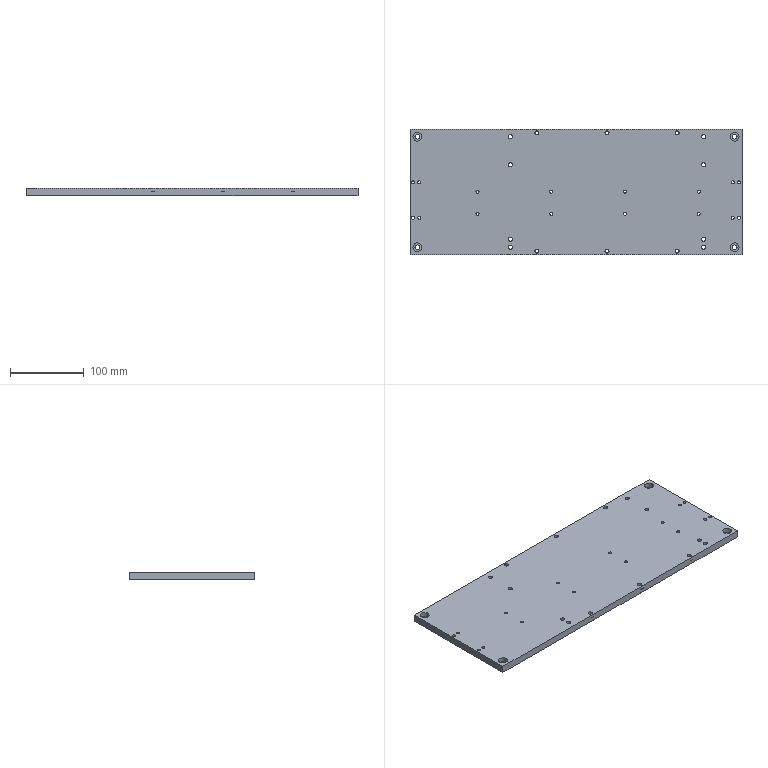Part | SolidWorks | features BaseBody 1 | 1 solid | 128 faces | box 450 x 170 x 10 mm | volume 751937 mm3 | cylinder 104 | plane 24 | commonest cylinder face diameters 5.5 x28 10 x28 4.134 x24 4 x8 6.5 x8 12 x8